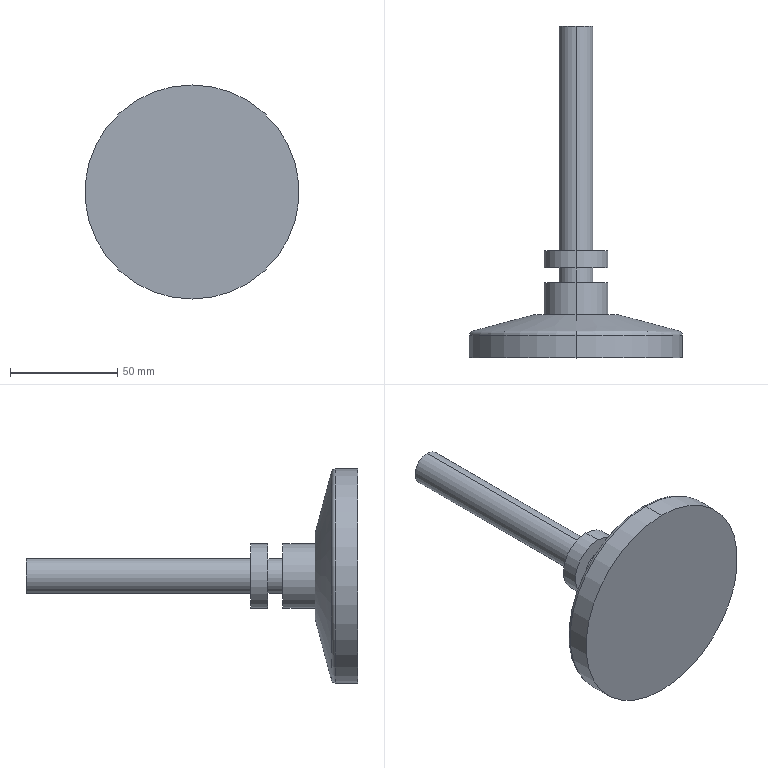Part | STEP file | M16 cup foot | 1 solid | 20 faces | box 100 x 155 x 100 mm | volume 165556 mm3 | cylinder 10 | plane 6 | torus 2 | cone 2 | commonest cylinder face diameters 16 x4 30 x4 100 x2
STEP:
#1=CARTESIAN_POINT('',(0.,0.,0.));
#2=DIRECTION('',(0.,0.,1.));
#3=DIRECTION('',(1.,0.,0.));
#4=AXIS2_PLACEMENT_3D('',#1,#2,#3);
#5=CARTESIAN_POINT('',(0.,120.,8.));
#6=VERTEX_POINT('',#5);
#7=CARTESIAN_POINT('',(0.,120.,-8.));
#8=VERTEX_POINT('',#7);
#9=CARTESIAN_POINT('',(0.,120.,0.));
#10=DIRECTION('',(0.,1.,0.));
#11=DIRECTION('',(0.,0.,1.));
#12=AXIS2_PLACEMENT_3D('',#9,#10,#11);
#13=CIRCLE('',#12,8.);
#14=CARTESIAN_POINT('',(0.,120.,0.));
#15=DIRECTION('',(0.,-1.,0.));
#16=DIRECTION('',(0.,0.,-1.));
#17=AXIS2_PLACEMENT_3D('',#14,#15,#16);
#18=CYLINDRICAL_SURFACE('',#17,8.);
#19=CARTESIAN_POINT('',(3.142,0.));
#20=DIRECTION('',(-1.,0.));
#21=VECTOR('',#20,1.);
#22=LINE('',#19,#21);
#23=(GEOMETRIC_REPRESENTATION_CONTEXT(2)PARAMETRIC_REPRESENTATION_CONTEXT()REPRESENTATION_CONTEXT('',''));
#24=DEFINITIONAL_REPRESENTATION('',(#22),#23);
#25=PCURVE('',#18,#24);
#26=CARTESIAN_POINT('',(0.,120.,0.));
#27=DIRECTION('',(0.,1.,0.));
#28=DIRECTION('',(0.,0.,1.));
#29=AXIS2_PLACEMENT_3D('',#26,#27,#28);
#30=PLANE('',#29);
#31=CARTESIAN_POINT('',(0.,0.));
#32=DIRECTION('',(1.,0.));
#33=AXIS2_PLACEMENT_2D('',#31,#32);
#34=CIRCLE('',#33,8.);
#35=(GEOMETRIC_REPRESENTATION_CONTEXT(2)PARAMETRIC_REPRESENTATION_CONTEXT()REPRESENTATION_CONTEXT('',''));
#36=DEFINITIONAL_REPRESENTATION('',(#34),#35);
#37=PCURVE('',#30,#36);
#38=SURFACE_CURVE('',#13,(#25,#37),.PCURVE_S1.);
#39=EDGE_CURVE('',#6,#8,#38,.T.);
#40=ORIENTED_EDGE('',*,*,#39,.F.);
#41=CARTESIAN_POINT('',(0.,15.,8.));
#42=VERTEX_POINT('',#41);
#43=CARTESIAN_POINT('',(0.,120.,8.));
#44=DIRECTION('',(0.,-1.,0.));
#45=VECTOR('',#44,1.);
#46=LINE('',#43,#45);
#47=CARTESIAN_POINT('',(3.142,0.));
#48=DIRECTION('',(0.,1.));
#49=VECTOR('',#48,1.);
#50=LINE('',#47,#49);
#51=(GEOMETRIC_REPRESENTATION_CONTEXT(2)PARAMETRIC_REPRESENTATION_CONTEXT()REPRESENTATION_CONTEXT('',''));
#52=DEFINITIONAL_REPRESENTATION('',(#50),#51);
#53=PCURVE('',#18,#52);
#54=CARTESIAN_POINT('',(0.,120.,0.));
#55=DIRECTION('',(0.,-1.,0.));
#56=DIRECTION('',(0.,0.,-1.));
#57=AXIS2_PLACEMENT_3D('',#54,#55,#56);
#58=CYLINDRICAL_SURFACE('',#57,8.);
#59=CARTESIAN_POINT('',(3.142,0.));
#60=DIRECTION('',(0.,1.));
#61=VECTOR('',#60,1.);
#62=LINE('',#59,#61);
#63=(GEOMETRIC_REPRESENTATION_CONTEXT(2)PARAMETRIC_REPRESENTATION_CONTEXT()REPRESENTATION_CONTEXT('',''));
#64=DEFINITIONAL_REPRESENTATION('',(#62),#63);
#65=PCURVE('',#58,#64);
#66=SURFACE_CURVE('',#46,(#53,#65),.PCURVE_S1.);
#67=EDGE_CURVE('',#6,#42,#66,.T.);
#68=ORIENTED_EDGE('',*,*,#67,.T.);
#69=CARTESIAN_POINT('',(0.,15.,-8.));
#70=VERTEX_POINT('',#69);
#71=CARTESIAN_POINT('',(0.,15.,0.));
#72=DIRECTION('',(0.,-1.,0.));
#73=DIRECTION('',(0.,0.,-1.));
#74=AXIS2_PLACEMENT_3D('',#71,#72,#73);
#75=CIRCLE('',#74,8.);
#76=CARTESIAN_POINT('',(0.,105.));
#77=DIRECTION('',(1.,0.));
#78=VECTOR('',#77,1.);
#79=LINE('',#76,#78);
#80=(GEOMETRIC_REPRESENTATION_CONTEXT(2)PARAMETRIC_REPRESENTATION_CONTEXT()REPRESENTATION_CONTEXT('',''));
#81=DEFINITIONAL_REPRESENTATION('',(#79),#80);
#82=PCURVE('',#18,#81);
#83=CARTESIAN_POINT('',(0.,15.,0.));
#84=DIRECTION('',(0.,-1.,0.));
#85=DIRECTION('',(0.,0.,-1.));
#86=AXIS2_PLACEMENT_3D('',#83,#84,#85);
#87=PLANE('',#86);
#88=CARTESIAN_POINT('',(0.,0.));
#89=DIRECTION('',(1.,0.));
#90=AXIS2_PLACEMENT_2D('',#88,#89);
#91=CIRCLE('',#90,8.);
#92=(GEOMETRIC_REPRESENTATION_CONTEXT(2)PARAMETRIC_REPRESENTATION_CONTEXT()REPRESENTATION_CONTEXT('',''));
#93=DEFINITIONAL_REPRESENTATION('',(#91),#92);
#94=PCURVE('',#87,#93);
#95=SURFACE_CURVE('',#75,(#82,#94),.PCURVE_S1.);
#96=EDGE_CURVE('',#70,#42,#95,.T.);
#97=ORIENTED_EDGE('',*,*,#96,.F.);
#98=CARTESIAN_POINT('',(0.,120.,-8.));
#99=DIRECTION('',(0.,-1.,0.));
#100=VECTOR('',#99,1.);
#101=LINE('',#98,#100);
#102=CARTESIAN_POINT('',(0.,0.));
#103=DIRECTION('',(0.,1.));
#104=VECTOR('',#103,1.);
#105=LINE('',#102,#104);
#106=(GEOMETRIC_REPRESENTATION_CONTEXT(2)PARAMETRIC_REPRESENTATION_CONTEXT()REPRESENTATION_CONTEXT('',''));
#107=DEFINITIONAL_REPRESENTATION('',(#105),#106);
#108=PCURVE('',#18,#107);
#109=CARTESIAN_POINT('',(6.283,0.));
#110=DIRECTION('',(0.,1.));
#111=VECTOR('',#110,1.);
#112=LINE('',#109,#111);
#113=(GEOMETRIC_REPRESENTATION_CONTEXT(2)PARAMETRIC_REPRESENTATION_CONTEXT()REPRESENTATION_CONTEXT('',''));
#114=DEFINITIONAL_REPRESENTATION('',(#112),#113);
#115=PCURVE('',#58,#114);
#116=SURFACE_CURVE('',#101,(#108,#115),.PCURVE_S1.);
#117=EDGE_CURVE('',#8,#70,#116,.T.);
#118=ORIENTED_EDGE('',*,*,#117,.F.);
#119=EDGE_LOOP('',(#40,#68,#97,#118));
#120=FACE_BOUND('',#119,.T.);
#121=ADVANCED_FACE('',(#120),#18,.T.);
#122=CARTESIAN_POINT('',(0.,7.,-15.));
#123=VERTEX_POINT('',#122);
#124=CARTESIAN_POINT('',(0.,7.,15.));
#125=VERTEX_POINT('',#124);
#126=CARTESIAN_POINT('',(0.,7.,0.));
#127=DIRECTION('',(0.,-1.,0.));
#128=DIRECTION('',(0.,0.,-1.));
#129=AXIS2_PLACEMENT_3D('',#126,#127,#128);
#130=CIRCLE('',#129,15.);
#131=CARTESIAN_POINT('',(0.,7.,0.));
#132=DIRECTION('',(0.,1.,0.));
#133=DIRECTION('',(0.,0.,1.));
#134=AXIS2_PLACEMENT_3D('',#131,#132,#133);
#135=CYLINDRICAL_SURFACE('',#134,15.);
#136=CARTESIAN_POINT('',(3.142,0.));
#137=DIRECTION('',(-1.,0.));
#138=VECTOR('',#137,1.);
#139=LINE('',#136,#138);
#140=(GEOMETRIC_REPRESENTATION_CONTEXT(2)PARAMETRIC_REPRESENTATION_CONTEXT()REPRESENTATION_CONTEXT('',''));
#141=DEFINITIONAL_REPRESENTATION('',(#139),#140);
#142=PCURVE('',#135,#141);
#143=CARTESIAN_POINT('',(0.,7.,0.));
#144=DIRECTION('',(0.,-1.,0.));
#145=DIRECTION('',(0.,0.,-1.));
#146=AXIS2_PLACEMENT_3D('',#143,#144,#145);
#147=PLANE('',#146);
#148=CARTESIAN_POINT('',(0.,0.));
#149=DIRECTION('',(1.,0.));
#150=AXIS2_PLACEMENT_2D('',#148,#149);
#151=CIRCLE('',#150,15.);
#152=(GEOMETRIC_REPRESENTATION_CONTEXT(2)PARAMETRIC_REPRESENTATION_CONTEXT()REPRESENTATION_CONTEXT('',''));
#153=DEFINITIONAL_REPRESENTATION('',(#151),#152);
#154=PCURVE('',#147,#153);
#155=SURFACE_CURVE('',#130,(#142,#154),.PCURVE_S1.);
#156=EDGE_CURVE('',#123,#125,#155,.T.);
#157=ORIENTED_EDGE('',*,*,#156,.F.);
#158=CARTESIAN_POINT('',(0.,15.,-15.));
#159=VERTEX_POINT('',#158);
#160=CARTESIAN_POINT('',(0.,7.,-15.));
#161=DIRECTION('',(0.,1.,0.));
#162=VECTOR('',#161,1.);
#163=LINE('',#160,#162);
#164=CARTESIAN_POINT('',(3.142,0.));
#165=DIRECTION('',(0.,1.));
#166=VECTOR('',#165,1.);
#167=LINE('',#164,#166);
#168=(GEOMETRIC_REPRESENTATION_CONTEXT(2)PARAMETRIC_REPRESENTATION_CONTEXT()REPRESENTATION_CONTEXT('',''));
#169=DEFINITIONAL_REPRESENTATION('',(#167),#168);
#170=PCURVE('',#135,#169);
#171=CARTESIAN_POINT('',(0.,7.,0.));
#172=DIRECTION('',(0.,1.,0.));
#173=DIRECTION('',(0.,0.,1.));
#174=AXIS2_PLACEMENT_3D('',#171,#172,#173);
#175=CYLINDRICAL_SURFACE('',#174,15.);
#176=CARTESIAN_POINT('',(3.142,0.));
#177=DIRECTION('',(0.,1.));
#178=VECTOR('',#177,1.);
#179=LINE('',#176,#178);
#180=(GEOMETRIC_REPRESENTATION_CONTEXT(2)PARAMETRIC_REPRESENTATION_CONTEXT()REPRESENTATION_CONTEXT('',''));
#181=DEFINITIONAL_REPRESENTATION('',(#179),#180);
#182=PCURVE('',#175,#181);
#183=SURFACE_CURVE('',#163,(#170,#182),.PCURVE_S1.);
#184=EDGE_CURVE('',#123,#159,#183,.T.);
#185=ORIENTED_EDGE('',*,*,#184,.T.);
#186=CARTESIAN_POINT('',(0.,15.,15.));
#187=VERTEX_POINT('',#186);
#188=CARTESIAN_POINT('',(0.,15.,0.));
#189=DIRECTION('',(0.,-1.,0.));
#190=DIRECTION('',(0.,0.,-1.));
#191=AXIS2_PLACEMENT_3D('',#188,#189,#190);
#192=CIRCLE('',#191,15.);
#193=CARTESIAN_POINT('',(3.142,8.));
#194=DIRECTION('',(-1.,0.));
#195=VECTOR('',#194,1.);
#196=LINE('',#193,#195);
#197=(GEOMETRIC_REPRESENTATION_CONTEXT(2)PARAMETRIC_REPRESENTATION_CONTEXT()REPRESENTATION_CONTEXT('',''));
#198=DEFINITIONAL_REPRESENTATION('',(#196),#197);
#199=PCURVE('',#135,#198);
#200=CARTESIAN_POINT('',(0.,0.));
#201=DIRECTION('',(1.,0.));
#202=AXIS2_PLACEMENT_2D('',#200,#201);
#203=CIRCLE('',#202,15.);
#204=(GEOMETRIC_REPRESENTATION_CONTEXT(2)PARAMETRIC_REPRESENTATION_CONTEXT()REPRESENTATION_CONTEXT('',''));
#205=DEFINITIONAL_REPRESENTATION('',(#203),#204);
#206=PCURVE('',#87,#205);
#207=SURFACE_CURVE('',#192,(#199,#206),.PCURVE_S1.);
#208=EDGE_CURVE('',#159,#187,#207,.T.);
#209=ORIENTED_EDGE('',*,*,#208,.T.);
#210=CARTESIAN_POINT('',(0.,7.,15.));
#211=DIRECTION('',(0.,1.,0.));
#212=VECTOR('',#211,1.);
#213=LINE('',#210,#212);
#214=CARTESIAN_POINT('',(0.,0.));
#215=DIRECTION('',(0.,1.));
#216=VECTOR('',#215,1.);
#217=LINE('',#214,#216);
#218=(GEOMETRIC_REPRESENTATION_CONTEXT(2)PARAMETRIC_REPRESENTATION_CONTEXT()REPRESENTATION_CONTEXT('',''));
#219=DEFINITIONAL_REPRESENTATION('',(#217),#218);
#220=PCURVE('',#135,#219);
#221=CARTESIAN_POINT('',(6.283,0.));
#222=DIRECTION('',(0.,1.));
#223=VECTOR('',#222,1.);
#224=LINE('',#221,#223);
#225=(GEOMETRIC_REPRESENTATION_CONTEXT(2)PARAMETRIC_REPRESENTATION_CONTEXT()REPRESENTATION_CONTEXT('',''));
#226=DEFINITIONAL_REPRESENTATION('',(#224),#225);
#227=PCURVE('',#175,#226);
#228=SURFACE_CURVE('',#213,(#220,#227),.PCURVE_S1.);
#229=EDGE_CURVE('',#125,#187,#228,.T.);
#230=ORIENTED_EDGE('',*,*,#229,.F.);
#231=EDGE_LOOP('',(#157,#185,#209,#230));
#232=FACE_BOUND('',#231,.T.);
#233=ADVANCED_FACE('',(#232),#135,.T.);
#234=CARTESIAN_POINT('',(0.,-24.537,-50.));
#235=VERTEX_POINT('',#234);
#236=CARTESIAN_POINT('',(0.,-24.537,50.));
#237=VERTEX_POINT('',#236);
#238=CARTESIAN_POINT('',(0.,-24.537,0.));
#239=DIRECTION('',(0.,-1.,0.));
#240=DIRECTION('',(0.,0.,1.));
#241=AXIS2_PLACEMENT_3D('',#238,#239,#240);
#242=CIRCLE('',#241,50.);
#243=CARTESIAN_POINT('',(0.,-24.537,0.));
#244=DIRECTION('',(0.,1.,0.));
#245=DIRECTION('',(0.,0.,1.));
#246=AXIS2_PLACEMENT_3D('',#243,#244,#245);
#247=TOROIDAL_SURFACE('',#246,48.,2.);
#248=CARTESIAN_POINT('',(6.283,0.));
#249=DIRECTION('',(-1.,0.));
#250=VECTOR('',#249,1.);
#251=LINE('',#248,#250);
#252=(GEOMETRIC_REPRESENTATION_CONTEXT(2)PARAMETRIC_REPRESENTATION_CONTEXT()REPRESENTATION_CONTEXT('',''));
#253=DEFINITIONAL_REPRESENTATION('',(#251),#252);
#254=PCURVE('',#247,#253);
#255=CARTESIAN_POINT('',(0.,-35.,0.));
#256=DIRECTION('',(0.,1.,0.));
#257=DIRECTION('',(0.,0.,1.));
#258=AXIS2_PLACEMENT_3D('',#255,#256,#257);
#259=CYLINDRICAL_SURFACE('',#258,50.);
#260=CARTESIAN_POINT('',(6.283,10.463));
#261=DIRECTION('',(-1.,0.));
#262=VECTOR('',#261,1.);
#263=LINE('',#260,#262);
#264=(GEOMETRIC_REPRESENTATION_CONTEXT(2)PARAMETRIC_REPRESENTATION_CONTEXT()REPRESENTATION_CONTEXT('',''));
#265=DEFINITIONAL_REPRESENTATION('',(#263),#264);
#266=PCURVE('',#259,#265);
#267=SURFACE_CURVE('',#242,(#254,#266),.PCURVE_S1.);
#268=EDGE_CURVE('',#235,#237,#267,.T.);
#269=ORIENTED_EDGE('',*,*,#268,.F.);
#270=CARTESIAN_POINT('',(0.,-22.604,-48.515));
#271=VERTEX_POINT('',#270);
#272=CARTESIAN_POINT('',(0.,-24.537,-48.));
#273=DIRECTION('',(1.,0.,0.));
#274=DIRECTION('',(0.,0.,-1.));
#275=AXIS2_PLACEMENT_3D('',#272,#273,#274);
#276=CIRCLE('',#275,2.);
#277=CARTESIAN_POINT('',(3.142,0.));
#278=DIRECTION('',(0.,1.));
#279=VECTOR('',#278,1.);
#280=LINE('',#277,#279);
#281=(GEOMETRIC_REPRESENTATION_CONTEXT(2)PARAMETRIC_REPRESENTATION_CONTEXT()REPRESENTATION_CONTEXT('',''));
#282=DEFINITIONAL_REPRESENTATION('',(#280),#281);
#283=PCURVE('',#247,#282);
#284=CARTESIAN_POINT('',(0.,-24.537,0.));
#285=DIRECTION('',(0.,1.,0.));
#286=DIRECTION('',(0.,0.,1.));
#287=AXIS2_PLACEMENT_3D('',#284,#285,#286);
#288=TOROIDAL_SURFACE('',#287,48.,2.);
#289=CARTESIAN_POINT('',(3.142,0.));
#290=DIRECTION('',(0.,1.));
#291=VECTOR('',#290,1.);
#292=LINE('',#289,#291);
#293=(GEOMETRIC_REPRESENTATION_CONTEXT(2)PARAMETRIC_REPRESENTATION_CONTEXT()REPRESENTATION_CONTEXT('',''));
#294=DEFINITIONAL_REPRESENTATION('',(#292),#293);
#295=PCURVE('',#288,#294);
#296=SURFACE_CURVE('',#276,(#283,#295),.PCURVE_S1.);
#297=EDGE_CURVE('',#235,#271,#296,.T.);
#298=ORIENTED_EDGE('',*,*,#297,.T.);
#299=CARTESIAN_POINT('',(0.,-22.604,48.515));
#300=VERTEX_POINT('',#299);
#301=CARTESIAN_POINT('',(0.,-22.604,0.));
#302=DIRECTION('',(0.,1.,0.));
#303=DIRECTION('',(0.,0.,-1.));
#304=AXIS2_PLACEMENT_3D('',#301,#302,#303);
#305=CIRCLE('',#304,48.515);
#306=CARTESIAN_POINT('',(-3.142,1.31));
#307=DIRECTION('',(1.,0.));
#308=VECTOR('',#307,1.);
#309=LINE('',#306,#308);
#310=(GEOMETRIC_REPRESENTATION_CONTEXT(2)PARAMETRIC_REPRESENTATION_CONTEXT()REPRESENTATION_CONTEXT('',''));
#311=DEFINITIONAL_REPRESENTATION('',(#309),#310);
#312=PCURVE('',#247,#311);
#313=CARTESIAN_POINT('',(0.,-23.,0.));
#314=DIRECTION('',(0.,-1.,0.));
#315=DIRECTION('',(0.,0.,-1.));
#316=AXIS2_PLACEMENT_3D('',#313,#314,#315);
#317=CONICAL_SURFACE('',#316,50.,1.31);
#318=CARTESIAN_POINT('',(6.283,-0.3959));
#319=DIRECTION('',(-1.,0.));
#320=VECTOR('',#319,1.);
#321=LINE('',#318,#320);
#322=(GEOMETRIC_REPRESENTATION_CONTEXT(2)PARAMETRIC_REPRESENTATION_CONTEXT()REPRESENTATION_CONTEXT('',''));
#323=DEFINITIONAL_REPRESENTATION('',(#321),#322);
#324=PCURVE('',#317,#323);
#325=SURFACE_CURVE('',#305,(#312,#324),.PCURVE_S1.);
#326=EDGE_CURVE('',#300,#271,#325,.T.);
#327=ORIENTED_EDGE('',*,*,#326,.F.);
#328=CARTESIAN_POINT('',(0.,-24.537,48.));
#329=DIRECTION('',(-1.,0.,0.));
#330=DIRECTION('',(0.,0.,1.));
#331=AXIS2_PLACEMENT_3D('',#328,#329,#330);
#332=CIRCLE('',#331,2.);
#333=CARTESIAN_POINT('',(0.,0.));
#334=DIRECTION('',(0.,1.));
#335=VECTOR('',#334,1.);
#336=LINE('',#333,#335);
#337=(GEOMETRIC_REPRESENTATION_CONTEXT(2)PARAMETRIC_REPRESENTATION_CONTEXT()REPRESENTATION_CONTEXT('',''));
#338=DEFINITIONAL_REPRESENTATION('',(#336),#337);
#339=PCURVE('',#247,#338);
#340=CARTESIAN_POINT('',(6.283,0.));
#341=DIRECTION('',(0.,1.));
#342=VECTOR('',#341,1.);
#343=LINE('',#340,#342);
#344=(GEOMETRIC_REPRESENTATION_CONTEXT(2)PARAMETRIC_REPRESENTATION_CONTEXT()REPRESENTATION_CONTEXT('',''));
#345=DEFINITIONAL_REPRESENTATION('',(#343),#344);
#346=PCURVE('',#288,#345);
#347=SURFACE_CURVE('',#332,(#339,#346),.PCURVE_S1.);
#348=EDGE_CURVE('',#237,#300,#347,.T.);
#349=ORIENTED_EDGE('',*,*,#348,.F.);
#350=EDGE_LOOP('',(#269,#298,#327,#349));
#351=FACE_BOUND('',#350,.T.);
#352=ADVANCED_FACE('',(#351),#247,.T.);
#353=CARTESIAN_POINT('',(0.,-15.,20.));
#354=VERTEX_POINT('',#353);
#355=CARTESIAN_POINT('',(0.,-15.,-20.));
#356=VERTEX_POINT('',#355);
#357=CARTESIAN_POINT('',(0.,-15.,0.));
#358=DIRECTION('',(0.,1.,0.));
#359=DIRECTION('',(0.,0.,-1.));
#360=AXIS2_PLACEMENT_3D('',#357,#358,#359);
#361=CIRCLE('',#360,20.);
#362=CARTESIAN_POINT('',(6.283,-8.));
#363=DIRECTION('',(-1.,0.));
#364=VECTOR('',#363,1.);
#365=LINE('',#362,#364);
#366=(GEOMETRIC_REPRESENTATION_CONTEXT(2)PARAMETRIC_REPRESENTATION_CONTEXT()REPRESENTATION_CONTEXT('',''));
#367=DEFINITIONAL_REPRESENTATION('',(#365),#366);
#368=PCURVE('',#317,#367);
#369=CARTESIAN_POINT('',(0.,-15.,0.));
#370=DIRECTION('',(0.,-1.,0.));
#371=DIRECTION('',(0.,0.,-1.));
#372=AXIS2_PLACEMENT_3D('',#369,#370,#371);
#373=PLANE('',#372);
#374=CARTESIAN_POINT('',(20.,0.));
#375=CARTESIAN_POINT('',(20.,-34.641));
#376=CARTESIAN_POINT('',(-10.,-17.321));
#377=CARTESIAN_POINT('',(-40.,0.));
#378=CARTESIAN_POINT('',(-10.,17.321));
#379=CARTESIAN_POINT('',(20.,34.641));
#380=CARTESIAN_POINT('',(20.,0.));
#381=(BOUNDED_CURVE()B_SPLINE_CURVE(2,(#374,#375,#376,#377,#378,#379,#380),.UNSPECIFIED.,.T.,.F.)B_SPLINE_CURVE_WITH_KNOTS((1,2,2,2,2,1),(-2.094,0.,2.094,4.189,6.283,8.378),.UNSPECIFIED.)CURVE()GEOMETRIC_REPRESENTATION_ITEM()RATIONAL_B_SPLINE_CURVE((1.,0.5,1.,0.5,1.,0.5,1.))REPRESENTATION_ITEM(''));
#382=(GEOMETRIC_REPRESENTATION_CONTEXT(2)PARAMETRIC_REPRESENTATION_CONTEXT()REPRESENTATION_CONTEXT('',''));
#383=DEFINITIONAL_REPRESENTATION('',(#381),#382);
#384=PCURVE('',#373,#383);
#385=SURFACE_CURVE('',#361,(#368,#384),.PCURVE_S1.);
#386=EDGE_CURVE('',#354,#356,#385,.T.);
#387=ORIENTED_EDGE('',*,*,#386,.F.);
#388=CARTESIAN_POINT('',(0.,-23.,50.));
#389=DIRECTION('',(0.,-0.2577,0.9662));
#390=VECTOR('',#389,1.);
#391=LINE('',#388,#390);
#392=CARTESIAN_POINT('',(3.142,0.));
#393=DIRECTION('',(0.,1.));
#394=VECTOR('',#393,1.);
#395=LINE('',#392,#394);
#396=(GEOMETRIC_REPRESENTATION_CONTEXT(2)PARAMETRIC_REPRESENTATION_CONTEXT()REPRESENTATION_CONTEXT('',''));
#397=DEFINITIONAL_REPRESENTATION('',(#395),#396);
#398=PCURVE('',#317,#397);
#399=CARTESIAN_POINT('',(0.,-23.,0.));
#400=DIRECTION('',(0.,-1.,0.));
#401=DIRECTION('',(0.,0.,-1.));
#402=AXIS2_PLACEMENT_3D('',#399,#400,#401);
#403=CONICAL_SURFACE('',#402,50.,1.31);
#404=CARTESIAN_POINT('',(3.142,0.));
#405=DIRECTION('',(0.,1.));
#406=VECTOR('',#405,1.);
#407=LINE('',#404,#406);
#408=(GEOMETRIC_REPRESENTATION_CONTEXT(2)PARAMETRIC_REPRESENTATION_CONTEXT()REPRESENTATION_CONTEXT('',''));
#409=DEFINITIONAL_REPRESENTATION('',(#407),#408);
#410=PCURVE('',#403,#409);
#411=SURFACE_CURVE('',#391,(#398,#410),.PCURVE_S1.);
#412=EDGE_CURVE('',#354,#300,#411,.T.);
#413=ORIENTED_EDGE('',*,*,#412,.T.);
#414=ORIENTED_EDGE('',*,*,#326,.T.);
#415=CARTESIAN_POINT('',(0.,-23.,-50.));
#416=DIRECTION('',(0.,-0.2577,-0.9662));
#417=VECTOR('',#416,1.);
#418=LINE('',#415,#417);
#419=CARTESIAN_POINT('',(0.,0.));
#420=DIRECTION('',(0.,1.));
#421=VECTOR('',#420,1.);
#422=LINE('',#419,#421);
#423=(GEOMETRIC_REPRESENTATION_CONTEXT(2)PARAMETRIC_REPRESENTATION_CONTEXT()REPRESENTATION_CONTEXT('',''));
#424=DEFINITIONAL_REPRESENTATION('',(#422),#423);
#425=PCURVE('',#317,#424);
#426=CARTESIAN_POINT('',(6.283,0.));
#427=DIRECTION('',(0.,1.));
#428=VECTOR('',#427,1.);
#429=LINE('',#426,#428);
#430=(GEOMETRIC_REPRESENTATION_CONTEXT(2)PARAMETRIC_REPRESENTATION_CONTEXT()REPRESENTATION_CONTEXT('',''));
#431=DEFINITIONAL_REPRESENTATION('',(#429),#430);
#432=PCURVE('',#403,#431);
#433=SURFACE_CURVE('',#418,(#425,#432),.PCURVE_S1.);
#434=EDGE_CURVE('',#356,#271,#433,.T.);
#435=ORIENTED_EDGE('',*,*,#434,.F.);
#436=EDGE_LOOP('',(#387,#413,#414,#435));
#437=FACE_BOUND('',#436,.T.);
#438=ADVANCED_FACE('',(#437),#317,.T.);
#439=CARTESIAN_POINT('',(0.,-35.,-50.));
#440=VERTEX_POINT('',#439);
#441=CARTESIAN_POINT('',(0.,-35.,50.));
#442=VERTEX_POINT('',#441);
#443=CARTESIAN_POINT('',(0.,-35.,0.));
#444=DIRECTION('',(0.,-1.,0.));
#445=DIRECTION('',(0.,0.,-1.));
#446=AXIS2_PLACEMENT_3D('',#443,#444,#445);
#447=CIRCLE('',#446,50.);
#448=CARTESIAN_POINT('',(3.142,0.));
#449=DIRECTION('',(-1.,0.));
#450=VECTOR('',#449,1.);
#451=LINE('',#448,#450);
#452=(GEOMETRIC_REPRESENTATION_CONTEXT(2)PARAMETRIC_REPRESENTATION_CONTEXT()REPRESENTATION_CONTEXT('',''));
#453=DEFINITIONAL_REPRESENTATION('',(#451),#452);
#454=PCURVE('',#259,#453);
#455=CARTESIAN_POINT('',(0.,-35.,0.));
#456=DIRECTION('',(0.,-1.,0.));
#457=DIRECTION('',(0.,0.,-1.));
#458=AXIS2_PLACEMENT_3D('',#455,#456,#457);
#459=PLANE('',#458);
#460=CARTESIAN_POINT('',(0.,0.));
#461=DIRECTION('',(1.,0.));
#462=AXIS2_PLACEMENT_2D('',#460,#461);
#463=CIRCLE('',#462,50.);
#464=(GEOMETRIC_REPRESENTATION_CONTEXT(2)PARAMETRIC_REPRESENTATION_CONTEXT()REPRESENTATION_CONTEXT('',''));
#465=DEFINITIONAL_REPRESENTATION('',(#463),#464);
#466=PCURVE('',#459,#465);
#467=SURFACE_CURVE('',#447,(#454,#466),.PCURVE_S1.);
#468=EDGE_CURVE('',#440,#442,#467,.T.);
#469=ORIENTED_EDGE('',*,*,#468,.F.);
#470=CARTESIAN_POINT('',(0.,-35.,-50.));
#471=DIRECTION('',(0.,1.,0.));
#472=VECTOR('',#471,1.);
#473=LINE('',#470,#472);
#474=CARTESIAN_POINT('',(3.142,0.));
#475=DIRECTION('',(0.,1.));
#476=VECTOR('',#475,1.);
#477=LINE('',#474,#476);
#478=(GEOMETRIC_REPRESENTATION_CONTEXT(2)PARAMETRIC_REPRESENTATION_CONTEXT()REPRESENTATION_CONTEXT('',''));
#479=DEFINITIONAL_REPRESENTATION('',(#477),#478);
#480=PCURVE('',#259,#479);
#481=CARTESIAN_POINT('',(0.,-35.,0.));
#482=DIRECTION('',(0.,1.,0.));
#483=DIRECTION('',(0.,0.,1.));
#484=AXIS2_PLACEMENT_3D('',#481,#482,#483);
#485=CYLINDRICAL_SURFACE('',#484,50.);
#486=CARTESIAN_POINT('',(3.142,0.));
#487=DIRECTION('',(0.,1.));
#488=VECTOR('',#487,1.);
#489=LINE('',#486,#488);
#490=(GEOMETRIC_REPRESENTATION_CONTEXT(2)PARAMETRIC_REPRESENTATION_CONTEXT()REPRESENTATION_CONTEXT('',''));
#491=DEFINITIONAL_REPRESENTATION('',(#489),#490);
#492=PCURVE('',#485,#491);
#493=SURFACE_CURVE('',#473,(#480,#492),.PCURVE_S1.);
#494=EDGE_CURVE('',#440,#235,#493,.T.);
#495=ORIENTED_EDGE('',*,*,#494,.T.);
#496=ORIENTED_EDGE('',*,*,#268,.T.);
#497=CARTESIAN_POINT('',(0.,-35.,50.));
#498=DIRECTION('',(0.,1.,0.));
#499=VECTOR('',#498,1.);
#500=LINE('',#497,#499);
#501=CARTESIAN_POINT('',(0.,0.));
#502=DIRECTION('',(0.,1.));
#503=VECTOR('',#502,1.);
#504=LINE('',#501,#503);
#505=(GEOMETRIC_REPRESENTATION_CONTEXT(2)PARAMETRIC_REPRESENTATION_CONTEXT()REPRESENTATION_CONTEXT('',''));
#506=DEFINITIONAL_REPRESENTATION('',(#504),#505);
#507=PCURVE('',#259,#506);
#508=CARTESIAN_POINT('',(6.283,0.));
#509=DIRECTION('',(0.,1.));
#510=VECTOR('',#509,1.);
#511=LINE('',#508,#510);
#512=(GEOMETRIC_REPRESENTATION_CONTEXT(2)PARAMETRIC_REPRESENTATION_CONTEXT()REPRESENTATION_CONTEXT('',''));
#513=DEFINITIONAL_REPRESENTATION('',(#511),#512);
#514=PCURVE('',#485,#513);
#515=SURFACE_CURVE('',#500,(#507,#514),.PCURVE_S1.);
#516=EDGE_CURVE('',#442,#237,#515,.T.);
#517=ORIENTED_EDGE('',*,*,#516,.F.);
#518=EDGE_LOOP('',(#469,#495,#496,#517));
#519=FACE_BOUND('',#518,.T.);
#520=ADVANCED_FACE('',(#519),#259,.T.);
#521=CARTESIAN_POINT('',(0.,-15.,-15.));
#522=VERTEX_POINT('',#521);
#523=CARTESIAN_POINT('',(0.,-15.,15.));
#524=VERTEX_POINT('',#523);
#525=CARTESIAN_POINT('',(0.,-15.,0.));
#526=DIRECTION('',(0.,-1.,0.));
#527=DIRECTION('',(0.,0.,-1.));
#528=AXIS2_PLACEMENT_3D('',#525,#526,#527);
#529=CIRCLE('',#528,15.);
#530=CARTESIAN_POINT('',(0.,-15.,0.));
#531=DIRECTION('',(0.,1.,0.));
#532=DIRECTION('',(0.,0.,1.));
#533=AXIS2_PLACEMENT_3D('',#530,#531,#532);
#534=CYLINDRICAL_SURFACE('',#533,15.);
#535=CARTESIAN_POINT('',(3.142,0.));
#536=DIRECTION('',(-1.,0.));
#537=VECTOR('',#536,1.);
#538=LINE('',#535,#537);
#539=(GEOMETRIC_REPRESENTATION_CONTEXT(2)PARAMETRIC_REPRESENTATION_CONTEXT()REPRESENTATION_CONTEXT('',''));
#540=DEFINITIONAL_REPRESENTATION('',(#538),#539);
#541=PCURVE('',#534,#540);
#542=CARTESIAN_POINT('',(0.,0.));
#543=DIRECTION('',(1.,0.));
#544=AXIS2_PLACEMENT_2D('',#542,#543);
#545=CIRCLE('',#544,15.);
#546=(GEOMETRIC_REPRESENTATION_CONTEXT(2)PARAMETRIC_REPRESENTATION_CONTEXT()REPRESENTATION_CONTEXT('',''));
#547=DEFINITIONAL_REPRESENTATION('',(#545),#546);
#548=PCURVE('',#373,#547);
#549=SURFACE_CURVE('',#529,(#541,#548),.PCURVE_S1.);
#550=EDGE_CURVE('',#522,#524,#549,.T.);
#551=ORIENTED_EDGE('',*,*,#550,.F.);
#552=CARTESIAN_POINT('',(0.,0.,-15.));
#553=VERTEX_POINT('',#552);
#554=CARTESIAN_POINT('',(0.,-15.,-15.));
#555=DIRECTION('',(0.,1.,0.));
#556=VECTOR('',#555,1.);
#557=LINE('',#554,#556);
#558=CARTESIAN_POINT('',(3.142,0.));
#559=DIRECTION('',(0.,1.));
#560=VECTOR('',#559,1.);
#561=LINE('',#558,#560);
#562=(GEOMETRIC_REPRESENTATION_CONTEXT(2)PARAMETRIC_REPRESENTATION_CONTEXT()REPRESENTATION_CONTEXT('',''));
#563=DEFINITIONAL_REPRESENTATION('',(#561),#562);
#564=PCURVE('',#534,#563);
#565=CARTESIAN_POINT('',(0.,-15.,0.));
#566=DIRECTION('',(0.,1.,0.));
#567=DIRECTION('',(0.,0.,1.));
#568=AXIS2_PLACEMENT_3D('',#565,#566,#567);
#569=CYLINDRICAL_SURFACE('',#568,15.);
#570=CARTESIAN_POINT('',(3.142,0.));
#571=DIRECTION('',(0.,1.));
#572=VECTOR('',#571,1.);
#573=LINE('',#570,#572);
#574=(GEOMETRIC_REPRESENTATION_CONTEXT(2)PARAMETRIC_REPRESENTATION_CONTEXT()REPRESENTATION_CONTEXT('',''));
#575=DEFINITIONAL_REPRESENTATION('',(#573),#574);
#576=PCURVE('',#569,#575);
#577=SURFACE_CURVE('',#557,(#564,#576),.PCURVE_S1.);
#578=EDGE_CURVE('',#522,#553,#577,.T.);
#579=ORIENTED_EDGE('',*,*,#578,.T.);
#580=CARTESIAN_POINT('',(0.,0.,15.));
#581=VERTEX_POINT('',#580);
#582=CARTESIAN_POINT('',(0.,0.,0.));
#583=DIRECTION('',(0.,-1.,0.));
#584=DIRECTION('',(0.,0.,-1.));
#585=AXIS2_PLACEMENT_3D('',#582,#583,#584);
#586=CIRCLE('',#585,15.);
#587=CARTESIAN_POINT('',(3.142,15.));
#588=DIRECTION('',(-1.,0.));
#589=VECTOR('',#588,1.);
#590=LINE('',#587,#589);
#591=(GEOMETRIC_REPRESENTATION_CONTEXT(2)PARAMETRIC_REPRESENTATION_CONTEXT()REPRESENTATION_CONTEXT('',''));
#592=DEFINITIONAL_REPRESENTATION('',(#590),#591);
#593=PCURVE('',#534,#592);
#594=CARTESIAN_POINT('',(0.,0.,0.));
#595=DIRECTION('',(0.,-1.,0.));
#596=DIRECTION('',(0.,0.,-1.));
#597=AXIS2_PLACEMENT_3D('',#594,#595,#596);
#598=PLANE('',#597);
#599=CARTESIAN_POINT('',(0.,0.));
#600=DIRECTION('',(1.,0.));
#601=AXIS2_PLACEMENT_2D('',#599,#600);
#602=CIRCLE('',#601,15.);
#603=(GEOMETRIC_REPRESENTATION_CONTEXT(2)PARAMETRIC_REPRESENTATION_CONTEXT()REPRESENTATION_CONTEXT('',''));
#604=DEFINITIONAL_REPRESENTATION('',(#602),#603);
#605=PCURVE('',#598,#604);
#606=SURFACE_CURVE('',#586,(#593,#605),.PCURVE_S1.);
#607=EDGE_CURVE('',#553,#581,#606,.T.);
#608=ORIENTED_EDGE('',*,*,#607,.T.);
#609=CARTESIAN_POINT('',(0.,-15.,15.));
#610=DIRECTION('',(0.,1.,0.));
#611=VECTOR('',#610,1.);
#612=LINE('',#609,#611);
#613=CARTESIAN_POINT('',(0.,0.));
#614=DIRECTION('',(0.,1.));
#615=VECTOR('',#614,1.);
#616=LINE('',#613,#615);
#617=(GEOMETRIC_REPRESENTATION_CONTEXT(2)PARAMETRIC_REPRESENTATION_CONTEXT()REPRESENTATION_CONTEXT('',''));
#618=DEFINITIONAL_REPRESENTATION('',(#616),#617);
#619=PCURVE('',#534,#618);
#620=CARTESIAN_POINT('',(6.283,0.));
#621=DIRECTION('',(0.,1.));
#622=VECTOR('',#621,1.);
#623=LINE('',#620,#622);
#624=(GEOMETRIC_REPRESENTATION_CONTEXT(2)PARAMETRIC_REPRESENTATION_CONTEXT()REPRESENTATION_CONTEXT('',''));
#625=DEFINITIONAL_REPRESENTATION('',(#623),#624);
#626=PCURVE('',#569,#625);
#627=SURFACE_CURVE('',#612,(#619,#626),.PCURVE_S1.);
#628=EDGE_CURVE('',#524,#581,#627,.T.);
#629=ORIENTED_EDGE('',*,*,#628,.F.);
#630=EDGE_LOOP('',(#551,#579,#608,#629));
#631=FACE_BOUND('',#630,.T.);
#632=ADVANCED_FACE('',(#631),#534,.T.);
#633=CARTESIAN_POINT('',(0.,7.,-8.));
#634=VERTEX_POINT('',#633);
#635=CARTESIAN_POINT('',(0.,7.,8.));
#636=VERTEX_POINT('',#635);
#637=CARTESIAN_POINT('',(0.,7.,0.));
#638=DIRECTION('',(0.,-1.,0.));
#639=DIRECTION('',(0.,0.,-1.));
#640=AXIS2_PLACEMENT_3D('',#637,#638,#639);
#641=CIRCLE('',#640,8.);
#642=CARTESIAN_POINT('',(0.,120.,0.));
#643=DIRECTION('',(0.,-1.,0.));
#644=DIRECTION('',(0.,0.,-1.));
#645=AXIS2_PLACEMENT_3D('',#642,#643,#644);
#646=CYLINDRICAL_SURFACE('',#645,8.);
#647=CARTESIAN_POINT('',(0.,113.));
#648=DIRECTION('',(1.,0.));
#649=VECTOR('',#648,1.);
#650=LINE('',#647,#649);
#651=(GEOMETRIC_REPRESENTATION_CONTEXT(2)PARAMETRIC_REPRESENTATION_CONTEXT()REPRESENTATION_CONTEXT('',''));
#652=DEFINITIONAL_REPRESENTATION('',(#650),#651);
#653=PCURVE('',#646,#652);
#654=CARTESIAN_POINT('',(0.,0.));
#655=DIRECTION('',(1.,0.));
#656=AXIS2_PLACEMENT_2D('',#654,#655);
#657=CIRCLE('',#656,8.);
#658=(GEOMETRIC_REPRESENTATION_CONTEXT(2)PARAMETRIC_REPRESENTATION_CONTEXT()REPRESENTATION_CONTEXT('',''));
#659=DEFINITIONAL_REPRESENTATION('',(#657),#658);
#660=PCURVE('',#147,#659);
#661=SURFACE_CURVE('',#641,(#653,#660),.PCURVE_S1.);
#662=EDGE_CURVE('',#634,#636,#661,.T.);
#663=ORIENTED_EDGE('',*,*,#662,.T.);
#664=CARTESIAN_POINT('',(0.,0.,8.));
#665=VERTEX_POINT('',#664);
#666=CARTESIAN_POINT('',(0.,120.,8.));
#667=DIRECTION('',(0.,-1.,0.));
#668=VECTOR('',#667,1.);
#669=LINE('',#666,#668);
#670=CARTESIAN_POINT('',(3.142,0.));
#671=DIRECTION('',(0.,1.));
#672=VECTOR('',#671,1.);
#673=LINE('',#670,#672);
#674=(GEOMETRIC_REPRESENTATION_CONTEXT(2)PARAMETRIC_REPRESENTATION_CONTEXT()REPRESENTATION_CONTEXT('',''));
#675=DEFINITIONAL_REPRESENTATION('',(#673),#674);
#676=PCURVE('',#646,#675);
#677=CARTESIAN_POINT('',(0.,120.,0.));
#678=DIRECTION('',(0.,-1.,0.));
#679=DIRECTION('',(0.,0.,-1.));
#680=AXIS2_PLACEMENT_3D('',#677,#678,#679);
#681=CYLINDRICAL_SURFACE('',#680,8.);
#682=CARTESIAN_POINT('',(3.142,0.));
#683=DIRECTION('',(0.,1.));
#684=VECTOR('',#683,1.);
#685=LINE('',#682,#684);
#686=(GEOMETRIC_REPRESENTATION_CONTEXT(2)PARAMETRIC_REPRESENTATION_CONTEXT()REPRESENTATION_CONTEXT('',''));
#687=DEFINITIONAL_REPRESENTATION('',(#685),#686);
#688=PCURVE('',#681,#687);
#689=SURFACE_CURVE('',#669,(#676,#688),.PCURVE_S1.);
#690=EDGE_CURVE('',#636,#665,#689,.T.);
#691=ORIENTED_EDGE('',*,*,#690,.T.);
#692=CARTESIAN_POINT('',(0.,0.,-8.));
#693=VERTEX_POINT('',#692);
#694=CARTESIAN_POINT('',(0.,0.,0.));
#695=DIRECTION('',(0.,-1.,0.));
#696=DIRECTION('',(0.,0.,-1.));
#697=AXIS2_PLACEMENT_3D('',#694,#695,#696);
#698=CIRCLE('',#697,8.);
#699=CARTESIAN_POINT('',(0.,120.));
#700=DIRECTION('',(1.,0.));
#701=VECTOR('',#700,1.);
#702=LINE('',#699,#701);
#703=(GEOMETRIC_REPRESENTATION_CONTEXT(2)PARAMETRIC_REPRESENTATION_CONTEXT()REPRESENTATION_CONTEXT('',''));
#704=DEFINITIONAL_REPRESENTATION('',(#702),#703);
#705=PCURVE('',#646,#704);
#706=CARTESIAN_POINT('',(0.,0.));
#707=DIRECTION('',(1.,0.));
#708=AXIS2_PLACEMENT_2D('',#706,#707);
#709=CIRCLE('',#708,8.);
#710=(GEOMETRIC_REPRESENTATION_CONTEXT(2)PARAMETRIC_REPRESENTATION_CONTEXT()REPRESENTATION_CONTEXT('',''));
#711=DEFINITIONAL_REPRESENTATION('',(#709),#710);
#712=PCURVE('',#598,#711);
#713=SURFACE_CURVE('',#698,(#705,#712),.PCURVE_S1.);
#714=EDGE_CURVE('',#693,#665,#713,.T.);
#715=ORIENTED_EDGE('',*,*,#714,.F.);
#716=CARTESIAN_POINT('',(0.,120.,-8.));
#717=DIRECTION('',(0.,-1.,0.));
#718=VECTOR('',#717,1.);
#719=LINE('',#716,#718);
#720=CARTESIAN_POINT('',(0.,0.));
#721=DIRECTION('',(0.,1.));
#722=VECTOR('',#721,1.);
#723=LINE('',#720,#722);
#724=(GEOMETRIC_REPRESENTATION_CONTEXT(2)PARAMETRIC_REPRESENTATION_CONTEXT()REPRESENTATION_CONTEXT('',''));
#725=DEFINITIONAL_REPRESENTATION('',(#723),#724);
#726=PCURVE('',#646,#725);
#727=CARTESIAN_POINT('',(6.283,0.));
#728=DIRECTION('',(0.,1.));
#729=VECTOR('',#728,1.);
#730=LINE('',#727,#729);
#731=(GEOMETRIC_REPRESENTATION_CONTEXT(2)PARAMETRIC_REPRESENTATION_CONTEXT()REPRESENTATION_CONTEXT('',''));
#732=DEFINITIONAL_REPRESENTATION('',(#730),#731);
#733=PCURVE('',#681,#732);
#734=SURFACE_CURVE('',#719,(#726,#733),.PCURVE_S1.);
#735=EDGE_CURVE('',#634,#693,#734,.T.);
#736=ORIENTED_EDGE('',*,*,#735,.F.);
#737=EDGE_LOOP('',(#663,#691,#715,#736));
#738=FACE_BOUND('',#737,.T.);
#739=ADVANCED_FACE('',(#738),#646,.T.);
#740=ORIENTED_EDGE('',*,*,#690,.F.);
#741=CARTESIAN_POINT('',(0.,7.,0.));
#742=DIRECTION('',(0.,-1.,0.));
#743=DIRECTION('',(0.,0.,-1.));
#744=AXIS2_PLACEMENT_3D('',#741,#742,#743);
#745=CIRCLE('',#744,8.);
#746=CARTESIAN_POINT('',(0.,113.));
#747=DIRECTION('',(1.,0.));
#748=VECTOR('',#747,1.);
#749=LINE('',#746,#748);
#750=(GEOMETRIC_REPRESENTATION_CONTEXT(2)PARAMETRIC_REPRESENTATION_CONTEXT()REPRESENTATION_CONTEXT('',''));
#751=DEFINITIONAL_REPRESENTATION('',(#749),#750);
#752=PCURVE('',#681,#751);
#753=CARTESIAN_POINT('',(0.,0.));
#754=DIRECTION('',(1.,0.));
#755=AXIS2_PLACEMENT_2D('',#753,#754);
#756=CIRCLE('',#755,8.);
#757=(GEOMETRIC_REPRESENTATION_CONTEXT(2)PARAMETRIC_REPRESENTATION_CONTEXT()REPRESENTATION_CONTEXT('',''));
#758=DEFINITIONAL_REPRESENTATION('',(#756),#757);
#759=PCURVE('',#147,#758);
#760=SURFACE_CURVE('',#745,(#752,#759),.PCURVE_S1.);
#761=EDGE_CURVE('',#636,#634,#760,.T.);
#762=ORIENTED_EDGE('',*,*,#761,.T.);
#763=ORIENTED_EDGE('',*,*,#735,.T.);
#764=CARTESIAN_POINT('',(0.,0.,0.));
#765=DIRECTION('',(0.,-1.,0.));
#766=DIRECTION('',(0.,0.,-1.));
#767=AXIS2_PLACEMENT_3D('',#764,#765,#766);
#768=CIRCLE('',#767,8.);
#769=CARTESIAN_POINT('',(0.,120.));
#770=DIRECTION('',(1.,0.));
#771=VECTOR('',#770,1.);
#772=LINE('',#769,#771);
#773=(GEOMETRIC_REPRESENTATION_CONTEXT(2)PARAMETRIC_REPRESENTATION_CONTEXT()REPRESENTATION_CONTEXT('',''));
#774=DEFINITIONAL_REPRESENTATION('',(#772),#773);
#775=PCURVE('',#681,#774);
#776=CARTESIAN_POINT('',(0.,0.));
#777=DIRECTION('',(1.,0.));
#778=AXIS2_PLACEMENT_2D('',#776,#777);
#779=CIRCLE('',#778,8.);
#780=(GEOMETRIC_REPRESENTATION_CONTEXT(2)PARAMETRIC_REPRESENTATION_CONTEXT()REPRESENTATION_CONTEXT('',''));
#781=DEFINITIONAL_REPRESENTATION('',(#779),#780);
#782=PCURVE('',#598,#781);
#783=SURFACE_CURVE('',#768,(#775,#782),.PCURVE_S1.);
#784=EDGE_CURVE('',#665,#693,#783,.T.);
#785=ORIENTED_EDGE('',*,*,#784,.F.);
#786=EDGE_LOOP('',(#740,#762,#763,#785));
#787=FACE_BOUND('',#786,.T.);
#788=ADVANCED_FACE('',(#787),#681,.T.);
#789=CARTESIAN_POINT('',(0.,0.,0.));
#790=DIRECTION('',(0.,-1.,0.));
#791=DIRECTION('',(0.,0.,-1.));
#792=AXIS2_PLACEMENT_3D('',#789,#790,#791);
#793=CIRCLE('',#792,15.);
#794=CARTESIAN_POINT('',(0.,0.));
#795=DIRECTION('',(1.,0.));
#796=AXIS2_PLACEMENT_2D('',#794,#795);
#797=CIRCLE('',#796,15.);
#798=(GEOMETRIC_REPRESENTATION_CONTEXT(2)PARAMETRIC_REPRESENTATION_CONTEXT()REPRESENTATION_CONTEXT('',''));
#799=DEFINITIONAL_REPRESENTATION('',(#797),#798);
#800=PCURVE('',#598,#799);
#801=CARTESIAN_POINT('',(9.425,15.));
#802=DIRECTION('',(-1.,0.));
#803=VECTOR('',#802,1.);
#804=LINE('',#801,#803);
#805=(GEOMETRIC_REPRESENTATION_CONTEXT(2)PARAMETRIC_REPRESENTATION_CONTEXT()REPRESENTATION_CONTEXT('',''));
#806=DEFINITIONAL_REPRESENTATION('',(#804),#805);
#807=PCURVE('',#569,#806);
#808=SURFACE_CURVE('',#793,(#800,#807),.PCURVE_S1.);
#809=EDGE_CURVE('',#581,#553,#808,.T.);
#810=ORIENTED_EDGE('',*,*,#809,.F.);
#811=ORIENTED_EDGE('',*,*,#607,.F.);
#812=EDGE_LOOP('',(#810,#811));
#813=FACE_BOUND('',#812,.T.);
#814=ORIENTED_EDGE('',*,*,#714,.T.);
#815=ORIENTED_EDGE('',*,*,#784,.T.);
#816=EDGE_LOOP('',(#814,#815));
#817=FACE_BOUND('',#816,.T.);
#818=ADVANCED_FACE('',(#813,#817),#598,.F.);
#819=ORIENTED_EDGE('',*,*,#578,.F.);
#820=CARTESIAN_POINT('',(0.,-15.,0.));
#821=DIRECTION('',(0.,-1.,0.));
#822=DIRECTION('',(0.,0.,-1.));
#823=AXIS2_PLACEMENT_3D('',#820,#821,#822);
#824=CIRCLE('',#823,15.);
#825=CARTESIAN_POINT('',(9.425,0.));
#826=DIRECTION('',(-1.,0.));
#827=VECTOR('',#826,1.);
#828=LINE('',#825,#827);
#829=(GEOMETRIC_REPRESENTATION_CONTEXT(2)PARAMETRIC_REPRESENTATION_CONTEXT()REPRESENTATION_CONTEXT('',''));
#830=DEFINITIONAL_REPRESENTATION('',(#828),#829);
#831=PCURVE('',#569,#830);
#832=CARTESIAN_POINT('',(0.,0.));
#833=DIRECTION('',(1.,0.));
#834=AXIS2_PLACEMENT_2D('',#832,#833);
#835=CIRCLE('',#834,15.);
#836=(GEOMETRIC_REPRESENTATION_CONTEXT(2)PARAMETRIC_REPRESENTATION_CONTEXT()REPRESENTATION_CONTEXT('',''));
#837=DEFINITIONAL_REPRESENTATION('',(#835),#836);
#838=PCURVE('',#373,#837);
#839=SURFACE_CURVE('',#824,(#831,#838),.PCURVE_S1.);
#840=EDGE_CURVE('',#524,#522,#839,.T.);
#841=ORIENTED_EDGE('',*,*,#840,.F.);
#842=ORIENTED_EDGE('',*,*,#628,.T.);
#843=ORIENTED_EDGE('',*,*,#809,.T.);
#844=EDGE_LOOP('',(#819,#841,#842,#843));
#845=FACE_BOUND('',#844,.T.);
#846=ADVANCED_FACE('',(#845),#569,.T.);
#847=CARTESIAN_POINT('',(0.,-15.,0.));
#848=DIRECTION('',(0.,1.,0.));
#849=DIRECTION('',(0.,0.,-1.));
#850=AXIS2_PLACEMENT_3D('',#847,#848,#849);
#851=CIRCLE('',#850,20.);
#852=CARTESIAN_POINT('',(20.,0.));
#853=CARTESIAN_POINT('',(20.,-34.641));
#854=CARTESIAN_POINT('',(-10.,-17.321));
#855=CARTESIAN_POINT('',(-40.,0.));
#856=CARTESIAN_POINT('',(-10.,17.321));
#857=CARTESIAN_POINT('',(20.,34.641));
#858=CARTESIAN_POINT('',(20.,0.));
#859=(BOUNDED_CURVE()B_SPLINE_CURVE(2,(#852,#853,#854,#855,#856,#857,#858),.UNSPECIFIED.,.T.,.F.)B_SPLINE_CURVE_WITH_KNOTS((1,2,2,2,2,1),(-2.094,0.,2.094,4.189,6.283,8.378),.UNSPECIFIED.)CURVE()GEOMETRIC_REPRESENTATION_ITEM()RATIONAL_B_SPLINE_CURVE((1.,0.5,1.,0.5,1.,0.5,1.))REPRESENTATION_ITEM(''));
#860=(GEOMETRIC_REPRESENTATION_CONTEXT(2)PARAMETRIC_REPRESENTATION_CONTEXT()REPRESENTATION_CONTEXT('',''));
#861=DEFINITIONAL_REPRESENTATION('',(#859),#860);
#862=PCURVE('',#373,#861);
#863=CARTESIAN_POINT('',(6.283,-8.));
#864=DIRECTION('',(-1.,0.));
#865=VECTOR('',#864,1.);
#866=LINE('',#863,#865);
#867=(GEOMETRIC_REPRESENTATION_CONTEXT(2)PARAMETRIC_REPRESENTATION_CONTEXT()REPRESENTATION_CONTEXT('',''));
#868=DEFINITIONAL_REPRESENTATION('',(#866),#867);
#869=PCURVE('',#403,#868);
#870=SURFACE_CURVE('',#851,(#862,#869),.PCURVE_S1.);
#871=EDGE_CURVE('',#356,#354,#870,.T.);
#872=ORIENTED_EDGE('',*,*,#871,.T.);
#873=ORIENTED_EDGE('',*,*,#386,.T.);
#874=EDGE_LOOP('',(#872,#873));
#875=FACE_BOUND('',#874,.T.);
#876=ORIENTED_EDGE('',*,*,#840,.T.);
#877=ORIENTED_EDGE('',*,*,#550,.T.);
#878=EDGE_LOOP('',(#876,#877));
#879=FACE_BOUND('',#878,.T.);
#880=ADVANCED_FACE('',(#875,#879),#373,.F.);
#881=ORIENTED_EDGE('',*,*,#494,.F.);
#882=CARTESIAN_POINT('',(0.,-35.,0.));
#883=DIRECTION('',(0.,-1.,0.));
#884=DIRECTION('',(0.,0.,-1.));
#885=AXIS2_PLACEMENT_3D('',#882,#883,#884);
#886=CIRCLE('',#885,50.);
#887=CARTESIAN_POINT('',(9.425,0.));
#888=DIRECTION('',(-1.,0.));
#889=VECTOR('',#888,1.);
#890=LINE('',#887,#889);
#891=(GEOMETRIC_REPRESENTATION_CONTEXT(2)PARAMETRIC_REPRESENTATION_CONTEXT()REPRESENTATION_CONTEXT('',''));
#892=DEFINITIONAL_REPRESENTATION('',(#890),#891);
#893=PCURVE('',#485,#892);
#894=CARTESIAN_POINT('',(0.,0.));
#895=DIRECTION('',(1.,0.));
#896=AXIS2_PLACEMENT_2D('',#894,#895);
#897=CIRCLE('',#896,50.);
#898=(GEOMETRIC_REPRESENTATION_CONTEXT(2)PARAMETRIC_REPRESENTATION_CONTEXT()REPRESENTATION_CONTEXT('',''));
#899=DEFINITIONAL_REPRESENTATION('',(#897),#898);
#900=PCURVE('',#459,#899);
#901=SURFACE_CURVE('',#886,(#893,#900),.PCURVE_S1.);
#902=EDGE_CURVE('',#442,#440,#901,.T.);
#903=ORIENTED_EDGE('',*,*,#902,.F.);
#904=ORIENTED_EDGE('',*,*,#516,.T.);
#905=CARTESIAN_POINT('',(0.,-24.537,0.));
#906=DIRECTION('',(0.,-1.,0.));
#907=DIRECTION('',(0.,0.,1.));
#908=AXIS2_PLACEMENT_3D('',#905,#906,#907);
#909=CIRCLE('',#908,50.);
#910=CARTESIAN_POINT('',(6.283,10.463));
#911=DIRECTION('',(-1.,0.));
#912=VECTOR('',#911,1.);
#913=LINE('',#910,#912);
#914=(GEOMETRIC_REPRESENTATION_CONTEXT(2)PARAMETRIC_REPRESENTATION_CONTEXT()REPRESENTATION_CONTEXT('',''));
#915=DEFINITIONAL_REPRESENTATION('',(#913),#914);
#916=PCURVE('',#485,#915);
#917=CARTESIAN_POINT('',(6.283,0.));
#918=DIRECTION('',(-1.,0.));
#919=VECTOR('',#918,1.);
#920=LINE('',#917,#919);
#921=(GEOMETRIC_REPRESENTATION_CONTEXT(2)PARAMETRIC_REPRESENTATION_CONTEXT()REPRESENTATION_CONTEXT('',''));
#922=DEFINITIONAL_REPRESENTATION('',(#920),#921);
#923=PCURVE('',#288,#922);
#924=SURFACE_CURVE('',#909,(#916,#923),.PCURVE_S1.);
#925=EDGE_CURVE('',#237,#235,#924,.T.);
#926=ORIENTED_EDGE('',*,*,#925,.T.);
#927=EDGE_LOOP('',(#881,#903,#904,#926));
#928=FACE_BOUND('',#927,.T.);
#929=ADVANCED_FACE('',(#928),#485,.T.);
#930=ORIENTED_EDGE('',*,*,#902,.T.);
#931=ORIENTED_EDGE('',*,*,#468,.T.);
#932=EDGE_LOOP('',(#930,#931));
#933=FACE_BOUND('',#932,.T.);
#934=ADVANCED_FACE('',(#933),#459,.T.);
#935=ORIENTED_EDGE('',*,*,#412,.F.);
#936=ORIENTED_EDGE('',*,*,#871,.F.);
#937=ORIENTED_EDGE('',*,*,#434,.T.);
#938=CARTESIAN_POINT('',(0.,-22.604,0.));
#939=DIRECTION('',(0.,1.,0.));
#940=DIRECTION('',(0.,0.,-1.));
#941=AXIS2_PLACEMENT_3D('',#938,#939,#940);
#942=CIRCLE('',#941,48.515);
#943=CARTESIAN_POINT('',(6.283,-0.3959));
#944=DIRECTION('',(-1.,0.));
#945=VECTOR('',#944,1.);
#946=LINE('',#943,#945);
#947=(GEOMETRIC_REPRESENTATION_CONTEXT(2)PARAMETRIC_REPRESENTATION_CONTEXT()REPRESENTATION_CONTEXT('',''));
#948=DEFINITIONAL_REPRESENTATION('',(#946),#947);
#949=PCURVE('',#403,#948);
#950=CARTESIAN_POINT('',(3.142,1.31));
#951=DIRECTION('',(1.,0.));
#952=VECTOR('',#951,1.);
#953=LINE('',#950,#952);
#954=(GEOMETRIC_REPRESENTATION_CONTEXT(2)PARAMETRIC_REPRESENTATION_CONTEXT()REPRESENTATION_CONTEXT('',''));
#955=DEFINITIONAL_REPRESENTATION('',(#953),#954);
#956=PCURVE('',#288,#955);
#957=SURFACE_CURVE('',#942,(#949,#956),.PCURVE_S1.);
#958=EDGE_CURVE('',#271,#300,#957,.T.);
#959=ORIENTED_EDGE('',*,*,#958,.T.);
#960=EDGE_LOOP('',(#935,#936,#937,#959));
#961=FACE_BOUND('',#960,.T.);
#962=ADVANCED_FACE('',(#961),#403,.T.);
#963=ORIENTED_EDGE('',*,*,#297,.F.);
#964=ORIENTED_EDGE('',*,*,#925,.F.);
#965=ORIENTED_EDGE('',*,*,#348,.T.);
#966=ORIENTED_EDGE('',*,*,#958,.F.);
#967=EDGE_LOOP('',(#963,#964,#965,#966));
#968=FACE_BOUND('',#967,.T.);
#969=ADVANCED_FACE('',(#968),#288,.T.);
#970=CARTESIAN_POINT('',(0.,7.,0.));
#971=DIRECTION('',(0.,-1.,0.));
#972=DIRECTION('',(0.,0.,-1.));
#973=AXIS2_PLACEMENT_3D('',#970,#971,#972);
#974=CIRCLE('',#973,15.);
#975=CARTESIAN_POINT('',(0.,0.));
#976=DIRECTION('',(1.,0.));
#977=AXIS2_PLACEMENT_2D('',#975,#976);
#978=CIRCLE('',#977,15.);
#979=(GEOMETRIC_REPRESENTATION_CONTEXT(2)PARAMETRIC_REPRESENTATION_CONTEXT()REPRESENTATION_CONTEXT('',''));
#980=DEFINITIONAL_REPRESENTATION('',(#978),#979);
#981=PCURVE('',#147,#980);
#982=CARTESIAN_POINT('',(9.425,0.));
#983=DIRECTION('',(-1.,0.));
#984=VECTOR('',#983,1.);
#985=LINE('',#982,#984);
#986=(GEOMETRIC_REPRESENTATION_CONTEXT(2)PARAMETRIC_REPRESENTATION_CONTEXT()REPRESENTATION_CONTEXT('',''));
#987=DEFINITIONAL_REPRESENTATION('',(#985),#986);
#988=PCURVE('',#175,#987);
#989=SURFACE_CURVE('',#974,(#981,#988),.PCURVE_S1.);
#990=EDGE_CURVE('',#125,#123,#989,.T.);
#991=ORIENTED_EDGE('',*,*,#990,.T.);
#992=ORIENTED_EDGE('',*,*,#156,.T.);
#993=EDGE_LOOP('',(#991,#992));
#994=FACE_BOUND('',#993,.T.);
#995=ORIENTED_EDGE('',*,*,#662,.F.);
#996=ORIENTED_EDGE('',*,*,#761,.F.);
#997=EDGE_LOOP('',(#995,#996));
#998=FACE_BOUND('',#997,.T.);
#999=ADVANCED_FACE('',(#994,#998),#147,.T.);
#1000=CARTESIAN_POINT('',(0.,15.,0.));
#1001=DIRECTION('',(0.,-1.,0.));
#1002=DIRECTION('',(0.,0.,-1.));
#1003=AXIS2_PLACEMENT_3D('',#1000,#1001,#1002);
#1004=CIRCLE('',#1003,15.);
#1005=CARTESIAN_POINT('',(0.,0.));
#1006=DIRECTION('',(1.,0.));
#1007=AXIS2_PLACEMENT_2D('',#1005,#1006);
#1008=CIRCLE('',#1007,15.);
#1009=(GEOMETRIC_REPRESENTATION_CONTEXT(2)PARAMETRIC_REPRESENTATION_CONTEXT()REPRESENTATION_CONTEXT('',''));
#1010=DEFINITIONAL_REPRESENTATION('',(#1008),#1009);
#1011=PCURVE('',#87,#1010);
#1012=CARTESIAN_POINT('',(9.425,8.));
#1013=DIRECTION('',(-1.,0.));
#1014=VECTOR('',#1013,1.);
#1015=LINE('',#1012,#1014);
#1016=(GEOMETRIC_REPRESENTATION_CONTEXT(2)PARAMETRIC_REPRESENTATION_CONTEXT()REPRESENTATION_CONTEXT('',''));
#1017=DEFINITIONAL_REPRESENTATION('',(#1015),#1016);
#1018=PCURVE('',#175,#1017);
#1019=SURFACE_CURVE('',#1004,(#1011,#1018),.PCURVE_S1.);
#1020=EDGE_CURVE('',#187,#159,#1019,.T.);
#1021=ORIENTED_EDGE('',*,*,#1020,.F.);
#1022=ORIENTED_EDGE('',*,*,#208,.F.);
#1023=EDGE_LOOP('',(#1021,#1022));
#1024=FACE_BOUND('',#1023,.T.);
#1025=ORIENTED_EDGE('',*,*,#96,.T.);
#1026=CARTESIAN_POINT('',(0.,15.,0.));
#1027=DIRECTION('',(0.,-1.,0.));
#1028=DIRECTION('',(0.,0.,-1.));
#1029=AXIS2_PLACEMENT_3D('',#1026,#1027,#1028);
#1030=CIRCLE('',#1029,8.);
#1031=CARTESIAN_POINT('',(0.,0.));
#1032=DIRECTION('',(1.,0.));
#1033=AXIS2_PLACEMENT_2D('',#1031,#1032);
#1034=CIRCLE('',#1033,8.);
#1035=(GEOMETRIC_REPRESENTATION_CONTEXT(2)PARAMETRIC_REPRESENTATION_CONTEXT()REPRESENTATION_CONTEXT('',''));
#1036=DEFINITIONAL_REPRESENTATION('',(#1034),#1035);
#1037=PCURVE('',#87,#1036);
#1038=CARTESIAN_POINT('',(0.,105.));
#1039=DIRECTION('',(1.,0.));
#1040=VECTOR('',#1039,1.);
#1041=LINE('',#1038,#1040);
#1042=(GEOMETRIC_REPRESENTATION_CONTEXT(2)PARAMETRIC_REPRESENTATION_CONTEXT()REPRESENTATION_CONTEXT('',''));
#1043=DEFINITIONAL_REPRESENTATION('',(#1041),#1042);
#1044=PCURVE('',#58,#1043);
#1045=SURFACE_CURVE('',#1030,(#1037,#1044),.PCURVE_S1.);
#1046=EDGE_CURVE('',#42,#70,#1045,.T.);
#1047=ORIENTED_EDGE('',*,*,#1046,.T.);
#1048=EDGE_LOOP('',(#1025,#1047));
#1049=FACE_BOUND('',#1048,.T.);
#1050=ADVANCED_FACE('',(#1024,#1049),#87,.F.);
#1051=ORIENTED_EDGE('',*,*,#184,.F.);
#1052=ORIENTED_EDGE('',*,*,#990,.F.);
#1053=ORIENTED_EDGE('',*,*,#229,.T.);
#1054=ORIENTED_EDGE('',*,*,#1020,.T.);
#1055=EDGE_LOOP('',(#1051,#1052,#1053,#1054));
#1056=FACE_BOUND('',#1055,.T.);
#1057=ADVANCED_FACE('',(#1056),#175,.T.);
#1058=CARTESIAN_POINT('',(0.,120.,0.));
#1059=DIRECTION('',(0.,1.,0.));
#1060=DIRECTION('',(0.,0.,1.));
#1061=AXIS2_PLACEMENT_3D('',#1058,#1059,#1060);
#1062=CIRCLE('',#1061,8.);
#1063=CARTESIAN_POINT('',(0.,0.));
#1064=DIRECTION('',(1.,0.));
#1065=AXIS2_PLACEMENT_2D('',#1063,#1064);
#1066=CIRCLE('',#1065,8.);
#1067=(GEOMETRIC_REPRESENTATION_CONTEXT(2)PARAMETRIC_REPRESENTATION_CONTEXT()REPRESENTATION_CONTEXT('',''));
#1068=DEFINITIONAL_REPRESENTATION('',(#1066),#1067);
#1069=PCURVE('',#30,#1068);
#1070=CARTESIAN_POINT('',(9.425,0.));
#1071=DIRECTION('',(-1.,0.));
#1072=VECTOR('',#1071,1.);
#1073=LINE('',#1070,#1072);
#1074=(GEOMETRIC_REPRESENTATION_CONTEXT(2)PARAMETRIC_REPRESENTATION_CONTEXT()REPRESENTATION_CONTEXT('',''));
#1075=DEFINITIONAL_REPRESENTATION('',(#1073),#1074);
#1076=PCURVE('',#58,#1075);
#1077=SURFACE_CURVE('',#1062,(#1069,#1076),.PCURVE_S1.);
#1078=EDGE_CURVE('',#8,#6,#1077,.T.);
#1079=ORIENTED_EDGE('',*,*,#1078,.T.);
#1080=ORIENTED_EDGE('',*,*,#39,.T.);
#1081=EDGE_LOOP('',(#1079,#1080));
#1082=FACE_BOUND('',#1081,.T.);
#1083=ADVANCED_FACE('',(#1082),#30,.T.);
#1084=ORIENTED_EDGE('',*,*,#67,.F.);
#1085=ORIENTED_EDGE('',*,*,#1078,.F.);
#1086=ORIENTED_EDGE('',*,*,#117,.T.);
#1087=ORIENTED_EDGE('',*,*,#1046,.F.);
#1088=EDGE_LOOP('',(#1084,#1085,#1086,#1087));
#1089=FACE_BOUND('',#1088,.T.);
#1090=ADVANCED_FACE('',(#1089),#58,.T.);
#1091=CLOSED_SHELL('',(#121,#233,#352,#438,#520,#632,#739,#788,#818,#846,#880,#929,#934,#962,#969,#999,#1050,#1057,#1083,#1090));
#1092=MANIFOLD_SOLID_BREP('',#1091);
#1093=(LENGTH_UNIT()NAMED_UNIT(*)SI_UNIT(.MILLI.,.METRE.));
#1094=UNCERTAINTY_MEASURE_WITH_UNIT(LENGTH_MEASURE(0.0000001),#1093,'','');
#1095=(NAMED_UNIT(*)PLANE_ANGLE_UNIT()SI_UNIT($,.RADIAN.));
#1096=(NAMED_UNIT(*)SI_UNIT($,.STERADIAN.)SOLID_ANGLE_UNIT());
#1097=(GEOMETRIC_REPRESENTATION_CONTEXT(3)GLOBAL_UNCERTAINTY_ASSIGNED_CONTEXT((#1094))GLOBAL_UNIT_ASSIGNED_CONTEXT((#1093,#1095,#1096))REPRESENTATION_CONTEXT('',''));
#1098=ADVANCED_BREP_SHAPE_REPRESENTATION('',(#4,#1092),#1097);